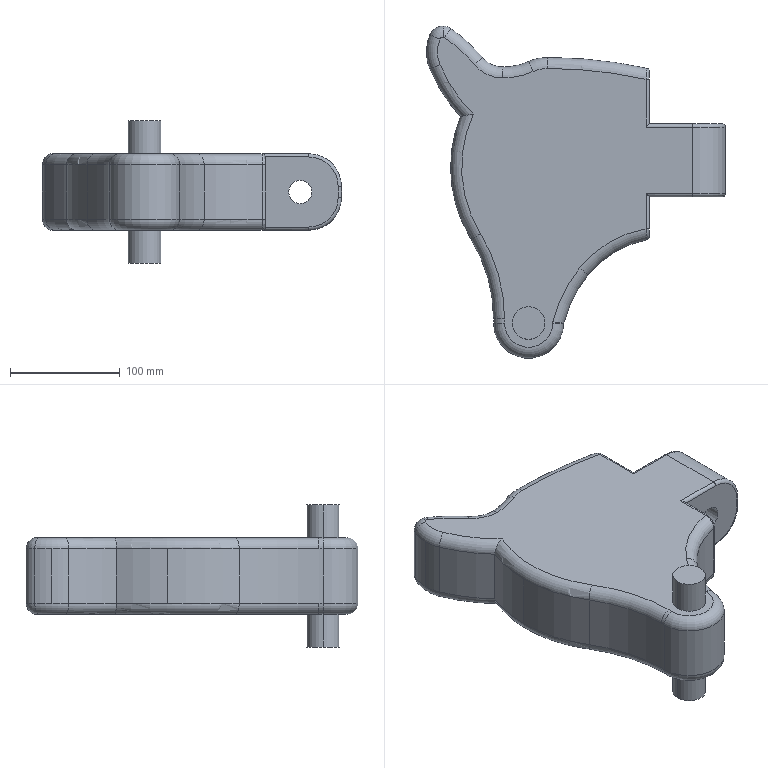Part | SolidWorks | features Fillet 3, ICE 3, Extrusion 1 | 1 solid | 91 faces | box 273.069 x 303.303 x 130 mm | volume 3030227 mm3 | cylinder 40 | torus 36 | plane 11 | spline 4 | commonest cylinder face diameters 6 x12 5.08 x4 29.973 x4 21.319 x2 60 x2 81.187 x2